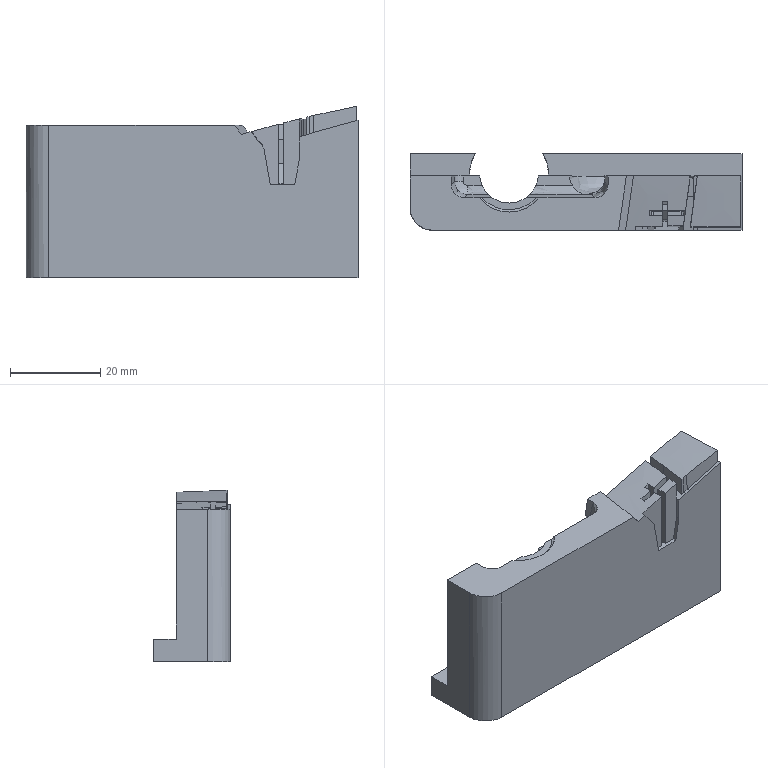Part | STEP file | P011002M008-000 | 1 solid | 84 faces | box 73.5 x 17 x 37.933 mm | volume 27742 mm3 | spline 48 | plane 28 | cylinder 6 | other 1 | cone 1 | commonest cylinder face diameters 1.012 x2 0.506 x1 10 x1 13 x1 17.5 x1